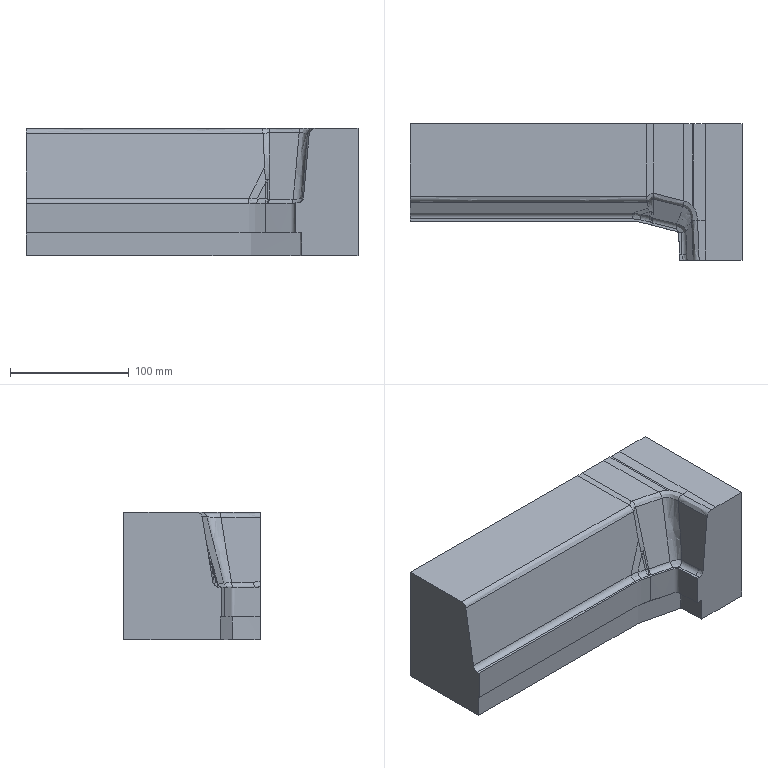Part | NX | features solid 2 | 1 solid | 55 faces | box 280 x 115 x 107.135 mm | volume 2442427 mm3 | spline 25 | plane 15 | cylinder 12 | cone 3 | commonest cylinder face diameters 12 x3 9 x2 10 x2 20 x2 8 x1 8.85 x1